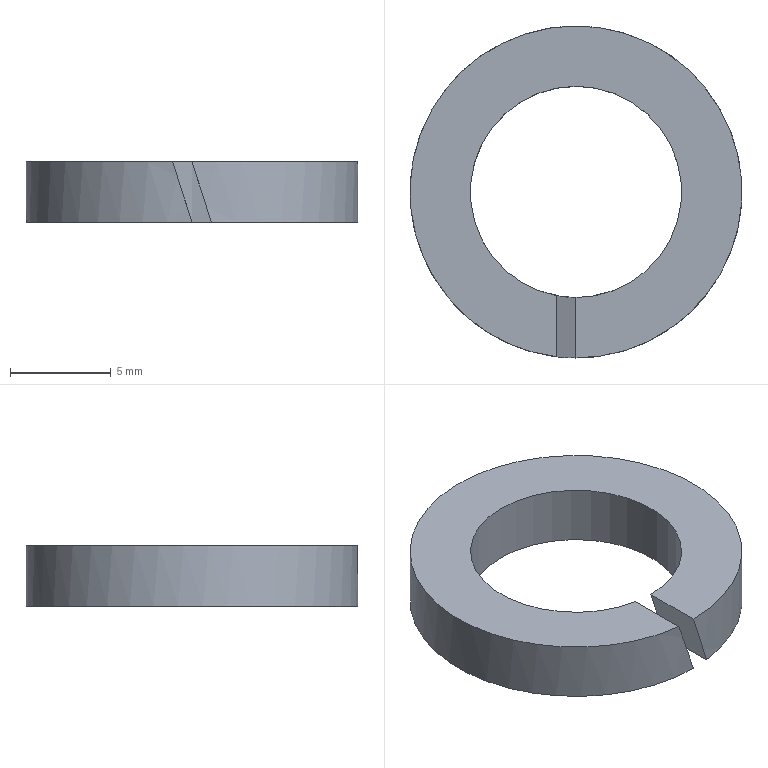Part | STEP file | 1_24 | 1 solid | 6 faces | box 16.5 x 16.5 x 3 mm | volume 372.946 mm3 | plane 4 | cylinder 2 | commonest cylinder face diameters 10.5 x1 16.5 x1
STEP:
#1=CARTESIAN_POINT('',(0.,0.,0.));
#2=DIRECTION('',(0.,0.,1.));
#3=DIRECTION('',(1.,0.,0.));
#4=AXIS2_PLACEMENT_3D('',#1,#2,#3);
#5=CARTESIAN_POINT('',(0.9706,-5.16,0.));
#6=VERTEX_POINT('',#5);
#7=CARTESIAN_POINT('',(0.,-5.25,3.));
#8=VERTEX_POINT('',#7);
#9=CARTESIAN_POINT('',(0.,0.,3.));
#10=DIRECTION('',(-0.9514,0.,-0.3078));
#11=DIRECTION('',(0.3078,0.,-0.9514));
#12=AXIS2_PLACEMENT_3D('',#9,#10,#11);
#13=ELLIPSE('',#12,17.055,5.25);
#14=CARTESIAN_POINT('',(0.,0.,1.5));
#15=DIRECTION('',(0.,0.,-1.));
#16=DIRECTION('',(1.,0.,0.));
#17=AXIS2_PLACEMENT_3D('',#14,#15,#16);
#18=CYLINDRICAL_SURFACE('',#17,5.25);
#19=CARTESIAN_POINT('',(7.668,1.5));
#20=CARTESIAN_POINT('',(7.854,-1.5));
#21=B_SPLINE_CURVE_WITH_KNOTS('',1,(#19,#20),.UNSPECIFIED.,.F.,.F.,(2,2),(1.385,1.571),.PIECEWISE_BEZIER_KNOTS.);
#22=(GEOMETRIC_REPRESENTATION_CONTEXT(2)PARAMETRIC_REPRESENTATION_CONTEXT()REPRESENTATION_CONTEXT('',''));
#23=DEFINITIONAL_REPRESENTATION('',(#21),#22);
#24=PCURVE('',#18,#23);
#25=CARTESIAN_POINT('',(0.,-4.95,3.));
#26=DIRECTION('',(0.9514,0.,0.3078));
#27=DIRECTION('',(0.3078,0.,-0.9514));
#28=AXIS2_PLACEMENT_3D('',#25,#26,#27);
#29=PLANE('',#28);
#30=CARTESIAN_POINT('',(17.055,4.95));
#31=CARTESIAN_POINT('',(17.055,-4.143));
#32=CARTESIAN_POINT('',(-8.528,0.4034));
#33=CARTESIAN_POINT('',(-34.111,4.95));
#34=CARTESIAN_POINT('',(-8.528,9.497));
#35=CARTESIAN_POINT('',(17.055,14.043));
#36=CARTESIAN_POINT('',(17.055,4.95));
#37=(BOUNDED_CURVE()B_SPLINE_CURVE(2,(#30,#31,#32,#33,#34,#35,#36),.UNSPECIFIED.,.T.,.F.)B_SPLINE_CURVE_WITH_KNOTS((1,2,2,2,2,1),(-2.094,0.,2.094,4.189,6.283,8.378),.UNSPECIFIED.)CURVE()GEOMETRIC_REPRESENTATION_ITEM()RATIONAL_B_SPLINE_CURVE((1.,0.5,1.,0.5,1.,0.5,1.))REPRESENTATION_ITEM(''));
#38=(GEOMETRIC_REPRESENTATION_CONTEXT(2)PARAMETRIC_REPRESENTATION_CONTEXT()REPRESENTATION_CONTEXT('',''));
#39=DEFINITIONAL_REPRESENTATION('',(#37),#38);
#40=PCURVE('',#29,#39);
#41=SURFACE_CURVE('',#13,(#24,#40),.PCURVE_S1.);
#42=EDGE_CURVE('',#6,#8,#41,.T.);
#43=ORIENTED_EDGE('',*,*,#42,.F.);
#44=CARTESIAN_POINT('',(0.,-5.25,0.));
#45=VERTEX_POINT('',#44);
#46=CARTESIAN_POINT('',(0.,0.,0.));
#47=DIRECTION('',(0.,0.,1.));
#48=DIRECTION('',(1.,0.,0.));
#49=AXIS2_PLACEMENT_3D('',#46,#47,#48);
#50=CIRCLE('',#49,5.25);
#51=CARTESIAN_POINT('',(12.566,1.5));
#52=DIRECTION('',(-1.,0.));
#53=VECTOR('',#52,1.);
#54=LINE('',#51,#53);
#55=(GEOMETRIC_REPRESENTATION_CONTEXT(2)PARAMETRIC_REPRESENTATION_CONTEXT()REPRESENTATION_CONTEXT('',''));
#56=DEFINITIONAL_REPRESENTATION('',(#54),#55);
#57=PCURVE('',#18,#56);
#58=CARTESIAN_POINT('',(6.75,0.,0.));
#59=DIRECTION('',(0.,0.,-1.));
#60=DIRECTION('',(-1.,0.,0.));
#61=AXIS2_PLACEMENT_3D('',#58,#59,#60);
#62=PLANE('',#61);
#63=CARTESIAN_POINT('',(1.5,0.));
#64=CARTESIAN_POINT('',(1.5,9.093));
#65=CARTESIAN_POINT('',(9.375,4.547));
#66=CARTESIAN_POINT('',(17.25,0.));
#67=CARTESIAN_POINT('',(9.375,-4.547));
#68=CARTESIAN_POINT('',(1.5,-9.093));
#69=CARTESIAN_POINT('',(1.5,0.));
#70=(BOUNDED_CURVE()B_SPLINE_CURVE(2,(#63,#64,#65,#66,#67,#68,#69),.UNSPECIFIED.,.T.,.F.)B_SPLINE_CURVE_WITH_KNOTS((1,2,2,2,2,1),(-2.094,0.,2.094,4.189,6.283,8.378),.UNSPECIFIED.)CURVE()GEOMETRIC_REPRESENTATION_ITEM()RATIONAL_B_SPLINE_CURVE((1.,0.5,1.,0.5,1.,0.5,1.))REPRESENTATION_ITEM(''));
#71=(GEOMETRIC_REPRESENTATION_CONTEXT(2)PARAMETRIC_REPRESENTATION_CONTEXT()REPRESENTATION_CONTEXT('',''));
#72=DEFINITIONAL_REPRESENTATION('',(#70),#71);
#73=PCURVE('',#62,#72);
#74=SURFACE_CURVE('',#50,(#57,#73),.PCURVE_S1.);
#75=EDGE_CURVE('',#6,#45,#74,.T.);
#76=ORIENTED_EDGE('',*,*,#75,.T.);
#77=CARTESIAN_POINT('',(-0.9706,-5.16,3.));
#78=VERTEX_POINT('',#77);
#79=CARTESIAN_POINT('',(0.,0.,0.));
#80=DIRECTION('',(0.9514,0.,0.3078));
#81=DIRECTION('',(0.3078,0.,-0.9514));
#82=AXIS2_PLACEMENT_3D('',#79,#80,#81);
#83=ELLIPSE('',#82,17.055,5.25);
#84=CARTESIAN_POINT('',(1.757,-1.5));
#85=CARTESIAN_POINT('',(1.571,1.5));
#86=B_SPLINE_CURVE_WITH_KNOTS('',1,(#84,#85),.UNSPECIFIED.,.F.,.F.,(2,2),(4.526,4.712),.PIECEWISE_BEZIER_KNOTS.);
#87=(GEOMETRIC_REPRESENTATION_CONTEXT(2)PARAMETRIC_REPRESENTATION_CONTEXT()REPRESENTATION_CONTEXT('',''));
#88=DEFINITIONAL_REPRESENTATION('',(#86),#87);
#89=PCURVE('',#18,#88);
#90=CARTESIAN_POINT('',(0.,-4.95,0.));
#91=DIRECTION('',(-0.9514,0.,-0.3078));
#92=DIRECTION('',(-0.3078,0.,0.9514));
#93=AXIS2_PLACEMENT_3D('',#90,#91,#92);
#94=PLANE('',#93);
#95=CARTESIAN_POINT('',(-17.055,4.95));
#96=CARTESIAN_POINT('',(-17.055,14.043));
#97=CARTESIAN_POINT('',(8.528,9.497));
#98=CARTESIAN_POINT('',(34.111,4.95));
#99=CARTESIAN_POINT('',(8.528,0.4034));
#100=CARTESIAN_POINT('',(-17.055,-4.143));
#101=CARTESIAN_POINT('',(-17.055,4.95));
#102=(BOUNDED_CURVE()B_SPLINE_CURVE(2,(#95,#96,#97,#98,#99,#100,#101),.UNSPECIFIED.,.T.,.F.)B_SPLINE_CURVE_WITH_KNOTS((1,2,2,2,2,1),(-2.094,0.,2.094,4.189,6.283,8.378),.UNSPECIFIED.)CURVE()GEOMETRIC_REPRESENTATION_ITEM()RATIONAL_B_SPLINE_CURVE((1.,0.5,1.,0.5,1.,0.5,1.))REPRESENTATION_ITEM(''));
#103=(GEOMETRIC_REPRESENTATION_CONTEXT(2)PARAMETRIC_REPRESENTATION_CONTEXT()REPRESENTATION_CONTEXT('',''));
#104=DEFINITIONAL_REPRESENTATION('',(#102),#103);
#105=PCURVE('',#94,#104);
#106=SURFACE_CURVE('',#83,(#89,#105),.PCURVE_S1.);
#107=EDGE_CURVE('',#78,#45,#106,.T.);
#108=ORIENTED_EDGE('',*,*,#107,.F.);
#109=CARTESIAN_POINT('',(0.,0.,3.));
#110=DIRECTION('',(0.,0.,-1.));
#111=DIRECTION('',(1.,0.,0.));
#112=AXIS2_PLACEMENT_3D('',#109,#110,#111);
#113=CIRCLE('',#112,5.25);
#114=CARTESIAN_POINT('',(0.,-1.5));
#115=DIRECTION('',(1.,0.));
#116=VECTOR('',#115,1.);
#117=LINE('',#114,#116);
#118=(GEOMETRIC_REPRESENTATION_CONTEXT(2)PARAMETRIC_REPRESENTATION_CONTEXT()REPRESENTATION_CONTEXT('',''));
#119=DEFINITIONAL_REPRESENTATION('',(#117),#118);
#120=PCURVE('',#18,#119);
#121=CARTESIAN_POINT('',(6.75,0.,3.));
#122=DIRECTION('',(0.,0.,1.));
#123=DIRECTION('',(1.,0.,0.));
#124=AXIS2_PLACEMENT_3D('',#121,#122,#123);
#125=PLANE('',#124);
#126=CARTESIAN_POINT('',(-1.5,0.));
#127=CARTESIAN_POINT('',(-1.5,-9.093));
#128=CARTESIAN_POINT('',(-9.375,-4.547));
#129=CARTESIAN_POINT('',(-17.25,0.));
#130=CARTESIAN_POINT('',(-9.375,4.547));
#131=CARTESIAN_POINT('',(-1.5,9.093));
#132=CARTESIAN_POINT('',(-1.5,0.));
#133=(BOUNDED_CURVE()B_SPLINE_CURVE(2,(#126,#127,#128,#129,#130,#131,#132),.UNSPECIFIED.,.T.,.F.)B_SPLINE_CURVE_WITH_KNOTS((1,2,2,2,2,1),(-2.094,0.,2.094,4.189,6.283,8.378),.UNSPECIFIED.)CURVE()GEOMETRIC_REPRESENTATION_ITEM()RATIONAL_B_SPLINE_CURVE((1.,0.5,1.,0.5,1.,0.5,1.))REPRESENTATION_ITEM(''));
#134=(GEOMETRIC_REPRESENTATION_CONTEXT(2)PARAMETRIC_REPRESENTATION_CONTEXT()REPRESENTATION_CONTEXT('',''));
#135=DEFINITIONAL_REPRESENTATION('',(#133),#134);
#136=PCURVE('',#125,#135);
#137=SURFACE_CURVE('',#113,(#120,#136),.PCURVE_S1.);
#138=EDGE_CURVE('',#78,#8,#137,.T.);
#139=ORIENTED_EDGE('',*,*,#138,.T.);
#140=EDGE_LOOP('',(#43,#76,#108,#139));
#141=FACE_BOUND('',#140,.F.);
#142=ADVANCED_FACE('',(#141),#18,.F.);
#143=CARTESIAN_POINT('',(0.,-8.25,3.));
#144=VERTEX_POINT('',#143);
#145=CARTESIAN_POINT('',(0.,-5.25,3.));
#146=DIRECTION('',(0.,-1.,0.));
#147=VECTOR('',#146,1.);
#148=LINE('',#145,#147);
#149=CARTESIAN_POINT('',(-6.75,-5.25));
#150=DIRECTION('',(0.,-1.));
#151=VECTOR('',#150,1.);
#152=LINE('',#149,#151);
#153=(GEOMETRIC_REPRESENTATION_CONTEXT(2)PARAMETRIC_REPRESENTATION_CONTEXT()REPRESENTATION_CONTEXT('',''));
#154=DEFINITIONAL_REPRESENTATION('',(#152),#153);
#155=PCURVE('',#125,#154);
#156=CARTESIAN_POINT('',(0.,-0.3));
#157=DIRECTION('',(0.,-1.));
#158=VECTOR('',#157,1.);
#159=LINE('',#156,#158);
#160=(GEOMETRIC_REPRESENTATION_CONTEXT(2)PARAMETRIC_REPRESENTATION_CONTEXT()REPRESENTATION_CONTEXT('',''));
#161=DEFINITIONAL_REPRESENTATION('',(#159),#160);
#162=PCURVE('',#29,#161);
#163=SURFACE_CURVE('',#148,(#155,#162),.PCURVE_S1.);
#164=EDGE_CURVE('',#8,#144,#163,.T.);
#165=ORIENTED_EDGE('',*,*,#164,.T.);
#166=CARTESIAN_POINT('',(-0.9706,-8.193,3.));
#167=VERTEX_POINT('',#166);
#168=CARTESIAN_POINT('',(0.000000003,-0.000000003,3.));
#169=DIRECTION('',(0.,0.,1.));
#170=DIRECTION('',(1.,0.,0.));
#171=AXIS2_PLACEMENT_3D('',#168,#169,#170);
#172=CIRCLE('',#171,8.25);
#173=CARTESIAN_POINT('',(-6.75,-0.000000003));
#174=DIRECTION('',(1.,0.));
#175=AXIS2_PLACEMENT_2D('',#173,#174);
#176=CIRCLE('',#175,8.25);
#177=(GEOMETRIC_REPRESENTATION_CONTEXT(2)PARAMETRIC_REPRESENTATION_CONTEXT()REPRESENTATION_CONTEXT('',''));
#178=DEFINITIONAL_REPRESENTATION('',(#176),#177);
#179=PCURVE('',#125,#178);
#180=CARTESIAN_POINT('',(0.,0.,1.5));
#181=DIRECTION('',(0.,0.,-1.));
#182=DIRECTION('',(1.,0.,0.));
#183=AXIS2_PLACEMENT_3D('',#180,#181,#182);
#184=CYLINDRICAL_SURFACE('',#183,8.25);
#185=CARTESIAN_POINT('',(12.566,-1.5));
#186=DIRECTION('',(-1.,0.));
#187=VECTOR('',#186,1.);
#188=LINE('',#185,#187);
#189=(GEOMETRIC_REPRESENTATION_CONTEXT(2)PARAMETRIC_REPRESENTATION_CONTEXT()REPRESENTATION_CONTEXT('',''));
#190=DEFINITIONAL_REPRESENTATION('',(#188),#189);
#191=PCURVE('',#184,#190);
#192=SURFACE_CURVE('',#172,(#179,#191),.PCURVE_S1.);
#193=EDGE_CURVE('',#144,#167,#192,.T.);
#194=ORIENTED_EDGE('',*,*,#193,.T.);
#195=CARTESIAN_POINT('',(-0.9706,-8.193,3.));
#196=DIRECTION('',(0.,1.,0.));
#197=VECTOR('',#196,1.);
#198=LINE('',#195,#197);
#199=CARTESIAN_POINT('',(-7.721,-8.193));
#200=DIRECTION('',(0.,1.));
#201=VECTOR('',#200,1.);
#202=LINE('',#199,#201);
#203=(GEOMETRIC_REPRESENTATION_CONTEXT(2)PARAMETRIC_REPRESENTATION_CONTEXT()REPRESENTATION_CONTEXT('',''));
#204=DEFINITIONAL_REPRESENTATION('',(#202),#203);
#205=PCURVE('',#125,#204);
#206=CARTESIAN_POINT('',(3.153,-3.243));
#207=DIRECTION('',(0.,1.));
#208=VECTOR('',#207,1.);
#209=LINE('',#206,#208);
#210=(GEOMETRIC_REPRESENTATION_CONTEXT(2)PARAMETRIC_REPRESENTATION_CONTEXT()REPRESENTATION_CONTEXT('',''));
#211=DEFINITIONAL_REPRESENTATION('',(#209),#210);
#212=PCURVE('',#94,#211);
#213=SURFACE_CURVE('',#198,(#205,#212),.PCURVE_S1.);
#214=EDGE_CURVE('',#167,#78,#213,.T.);
#215=ORIENTED_EDGE('',*,*,#214,.T.);
#216=ORIENTED_EDGE('',*,*,#138,.T.);
#217=EDGE_LOOP('',(#165,#194,#215,#216));
#218=FACE_BOUND('',#217,.T.);
#219=ADVANCED_FACE('',(#218),#125,.T.);
#220=ORIENTED_EDGE('',*,*,#107,.F.);
#221=ORIENTED_EDGE('',*,*,#214,.F.);
#222=CARTESIAN_POINT('',(0.,-8.25,0.));
#223=VERTEX_POINT('',#222);
#224=CARTESIAN_POINT('',(-0.01883,-0.319,0.0582));
#225=DIRECTION('',(-0.9514,0.,-0.3078));
#226=DIRECTION('',(0.3078,-0.0007728,-0.9514));
#227=AXIS2_PLACEMENT_3D('',#224,#225,#226);
#228=ELLIPSE('',#227,26.276,7.931);
#229=CARTESIAN_POINT('',(0.06117,4.631));
#230=DIRECTION('',(-1.,-0.0007728));
#231=AXIS2_PLACEMENT_2D('',#229,#230);
#232=ELLIPSE('',#231,26.276,7.931);
#233=(GEOMETRIC_REPRESENTATION_CONTEXT(2)PARAMETRIC_REPRESENTATION_CONTEXT()REPRESENTATION_CONTEXT('',''));
#234=DEFINITIONAL_REPRESENTATION('',(#232),#233);
#235=PCURVE('',#94,#234);
#236=CARTESIAN_POINT('',(1.571,1.5));
#237=CARTESIAN_POINT('',(1.689,-1.5));
#238=B_SPLINE_CURVE_WITH_KNOTS('',1,(#236,#237),.UNSPECIFIED.,.F.,.F.,(2,2),(1.568,1.689),.PIECEWISE_BEZIER_KNOTS.);
#239=(GEOMETRIC_REPRESENTATION_CONTEXT(2)PARAMETRIC_REPRESENTATION_CONTEXT()REPRESENTATION_CONTEXT('',''));
#240=DEFINITIONAL_REPRESENTATION('',(#238),#239);
#241=PCURVE('',#184,#240);
#242=SURFACE_CURVE('',#228,(#235,#241),.PCURVE_S1.);
#243=EDGE_CURVE('',#223,#167,#242,.T.);
#244=ORIENTED_EDGE('',*,*,#243,.F.);
#245=CARTESIAN_POINT('',(0.,-5.25,0.));
#246=DIRECTION('',(0.,-1.,0.));
#247=VECTOR('',#246,1.);
#248=LINE('',#245,#247);
#249=CARTESIAN_POINT('',(0.,-0.3));
#250=DIRECTION('',(0.,-1.));
#251=VECTOR('',#250,1.);
#252=LINE('',#249,#251);
#253=(GEOMETRIC_REPRESENTATION_CONTEXT(2)PARAMETRIC_REPRESENTATION_CONTEXT()REPRESENTATION_CONTEXT('',''));
#254=DEFINITIONAL_REPRESENTATION('',(#252),#253);
#255=PCURVE('',#94,#254);
#256=CARTESIAN_POINT('',(6.75,-5.25));
#257=DIRECTION('',(0.,-1.));
#258=VECTOR('',#257,1.);
#259=LINE('',#256,#258);
#260=(GEOMETRIC_REPRESENTATION_CONTEXT(2)PARAMETRIC_REPRESENTATION_CONTEXT()REPRESENTATION_CONTEXT('',''));
#261=DEFINITIONAL_REPRESENTATION('',(#259),#260);
#262=PCURVE('',#62,#261);
#263=SURFACE_CURVE('',#248,(#255,#262),.PCURVE_S1.);
#264=EDGE_CURVE('',#45,#223,#263,.T.);
#265=ORIENTED_EDGE('',*,*,#264,.F.);
#266=EDGE_LOOP('',(#220,#221,#244,#265));
#267=FACE_BOUND('',#266,.T.);
#268=ADVANCED_FACE('',(#267),#94,.F.);
#269=CARTESIAN_POINT('',(0.9706,-8.193,0.000000001));
#270=VERTEX_POINT('',#269);
#271=CARTESIAN_POINT('',(0.9706,-8.193,0.));
#272=DIRECTION('',(0.,1.,0.));
#273=VECTOR('',#272,1.);
#274=LINE('',#271,#273);
#275=CARTESIAN_POINT('',(5.779,-8.193));
#276=DIRECTION('',(0.,1.));
#277=VECTOR('',#276,1.);
#278=LINE('',#275,#277);
#279=(GEOMETRIC_REPRESENTATION_CONTEXT(2)PARAMETRIC_REPRESENTATION_CONTEXT()REPRESENTATION_CONTEXT('',''));
#280=DEFINITIONAL_REPRESENTATION('',(#278),#279);
#281=PCURVE('',#62,#280);
#282=CARTESIAN_POINT('',(3.153,-3.243));
#283=DIRECTION('',(0.,1.));
#284=VECTOR('',#283,1.);
#285=LINE('',#282,#284);
#286=(GEOMETRIC_REPRESENTATION_CONTEXT(2)PARAMETRIC_REPRESENTATION_CONTEXT()REPRESENTATION_CONTEXT('',''));
#287=DEFINITIONAL_REPRESENTATION('',(#285),#286);
#288=PCURVE('',#29,#287);
#289=SURFACE_CURVE('',#274,(#281,#288),.PCURVE_S1.);
#290=EDGE_CURVE('',#270,#6,#289,.T.);
#291=ORIENTED_EDGE('',*,*,#290,.T.);
#292=ORIENTED_EDGE('',*,*,#75,.T.);
#293=ORIENTED_EDGE('',*,*,#264,.T.);
#294=CARTESIAN_POINT('',(0.,0.,0.));
#295=DIRECTION('',(0.,0.,1.));
#296=DIRECTION('',(0.,-1.,0.));
#297=AXIS2_PLACEMENT_3D('',#294,#295,#296);
#298=CIRCLE('',#297,8.25);
#299=CARTESIAN_POINT('',(6.75,-8.25));
#300=CARTESIAN_POINT('',(-7.539,-8.25));
#301=CARTESIAN_POINT('',(-0.3947,4.125));
#302=CARTESIAN_POINT('',(6.75,16.5));
#303=CARTESIAN_POINT('',(13.895,4.125));
#304=CARTESIAN_POINT('',(21.039,-8.25));
#305=CARTESIAN_POINT('',(6.75,-8.25));
#306=(BOUNDED_CURVE()B_SPLINE_CURVE(2,(#299,#300,#301,#302,#303,#304,#305),.UNSPECIFIED.,.T.,.F.)B_SPLINE_CURVE_WITH_KNOTS((1,2,2,2,2,1),(-2.094,0.,2.094,4.189,6.283,8.378),.UNSPECIFIED.)CURVE()GEOMETRIC_REPRESENTATION_ITEM()RATIONAL_B_SPLINE_CURVE((1.,0.5,1.,0.5,1.,0.5,1.))REPRESENTATION_ITEM(''));
#307=(GEOMETRIC_REPRESENTATION_CONTEXT(2)PARAMETRIC_REPRESENTATION_CONTEXT()REPRESENTATION_CONTEXT('',''));
#308=DEFINITIONAL_REPRESENTATION('',(#306),#307);
#309=PCURVE('',#62,#308);
#310=CARTESIAN_POINT('',(7.854,1.5));
#311=DIRECTION('',(-1.,0.));
#312=VECTOR('',#311,1.);
#313=LINE('',#310,#312);
#314=(GEOMETRIC_REPRESENTATION_CONTEXT(2)PARAMETRIC_REPRESENTATION_CONTEXT()REPRESENTATION_CONTEXT('',''));
#315=DEFINITIONAL_REPRESENTATION('',(#313),#314);
#316=PCURVE('',#184,#315);
#317=SURFACE_CURVE('',#298,(#309,#316),.PCURVE_S1.);
#318=EDGE_CURVE('',#270,#223,#317,.T.);
#319=ORIENTED_EDGE('',*,*,#318,.F.);
#320=EDGE_LOOP('',(#291,#292,#293,#319));
#321=FACE_BOUND('',#320,.T.);
#322=ADVANCED_FACE('',(#321),#62,.T.);
#323=ORIENTED_EDGE('',*,*,#42,.F.);
#324=ORIENTED_EDGE('',*,*,#290,.F.);
#325=CARTESIAN_POINT('',(0.01883,-0.319,2.942));
#326=DIRECTION('',(0.9514,0.,0.3078));
#327=DIRECTION('',(0.3078,0.0007728,-0.9514));
#328=AXIS2_PLACEMENT_3D('',#325,#326,#327);
#329=ELLIPSE('',#328,26.276,7.931);
#330=CARTESIAN_POINT('',(0.06117,4.631));
#331=DIRECTION('',(1.,0.0007728));
#332=AXIS2_PLACEMENT_2D('',#330,#331);
#333=ELLIPSE('',#332,26.276,7.931);
#334=(GEOMETRIC_REPRESENTATION_CONTEXT(2)PARAMETRIC_REPRESENTATION_CONTEXT()REPRESENTATION_CONTEXT('',''));
#335=DEFINITIONAL_REPRESENTATION('',(#333),#334);
#336=PCURVE('',#29,#335);
#337=CARTESIAN_POINT('',(7.854,-1.5));
#338=CARTESIAN_POINT('',(7.736,1.5));
#339=B_SPLINE_CURVE_WITH_KNOTS('',1,(#337,#338),.UNSPECIFIED.,.F.,.F.,(2,2),(4.71,4.83),.PIECEWISE_BEZIER_KNOTS.);
#340=(GEOMETRIC_REPRESENTATION_CONTEXT(2)PARAMETRIC_REPRESENTATION_CONTEXT()REPRESENTATION_CONTEXT('',''));
#341=DEFINITIONAL_REPRESENTATION('',(#339),#340);
#342=PCURVE('',#184,#341);
#343=SURFACE_CURVE('',#329,(#336,#342),.PCURVE_S1.);
#344=EDGE_CURVE('',#144,#270,#343,.T.);
#345=ORIENTED_EDGE('',*,*,#344,.F.);
#346=ORIENTED_EDGE('',*,*,#164,.F.);
#347=EDGE_LOOP('',(#323,#324,#345,#346));
#348=FACE_BOUND('',#347,.T.);
#349=ADVANCED_FACE('',(#348),#29,.F.);
#350=ORIENTED_EDGE('',*,*,#193,.F.);
#351=ORIENTED_EDGE('',*,*,#344,.T.);
#352=ORIENTED_EDGE('',*,*,#318,.T.);
#353=ORIENTED_EDGE('',*,*,#243,.T.);
#354=EDGE_LOOP('',(#350,#351,#352,#353));
#355=FACE_BOUND('',#354,.T.);
#356=ADVANCED_FACE('',(#355),#184,.T.);
#357=CLOSED_SHELL('',(#142,#219,#268,#322,#349,#356));
#358=MANIFOLD_SOLID_BREP('',#357);
#359=(LENGTH_UNIT()NAMED_UNIT(*)SI_UNIT(.MILLI.,.METRE.));
#360=UNCERTAINTY_MEASURE_WITH_UNIT(LENGTH_MEASURE(0.005),#359,'','');
#361=(NAMED_UNIT(*)PLANE_ANGLE_UNIT()SI_UNIT($,.RADIAN.));
#362=(NAMED_UNIT(*)SI_UNIT($,.STERADIAN.)SOLID_ANGLE_UNIT());
#363=(GEOMETRIC_REPRESENTATION_CONTEXT(3)GLOBAL_UNCERTAINTY_ASSIGNED_CONTEXT((#360))GLOBAL_UNIT_ASSIGNED_CONTEXT((#359,#361,#362))REPRESENTATION_CONTEXT('',''));
#364=ADVANCED_BREP_SHAPE_REPRESENTATION('',(#4,#358),#363);